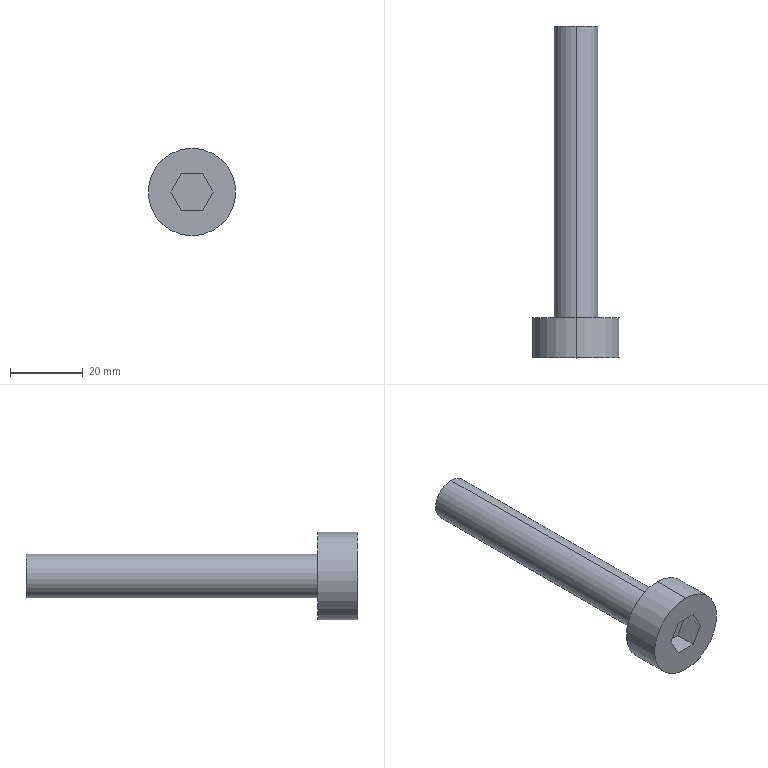Part | STEP file | PN_0057 (M12X60) | 1 solid | 14 faces | box 24 x 91 x 24 mm | volume 13504 mm3 | plane 10 | cylinder 4 | commonest cylinder face diameters 12 x2 24 x2
STEP:
#1=CARTESIAN_POINT('',(0.,0.,0.));
#2=DIRECTION('',(0.,0.,1.));
#3=DIRECTION('',(1.,0.,0.));
#4=AXIS2_PLACEMENT_3D('',#1,#2,#3);
#5=CARTESIAN_POINT('',(0.,91.,-6.));
#6=VERTEX_POINT('',#5);
#7=CARTESIAN_POINT('',(0.,91.,6.));
#8=VERTEX_POINT('',#7);
#9=CARTESIAN_POINT('',(0.,91.,0.));
#10=DIRECTION('',(0.,-1.,0.));
#11=DIRECTION('',(0.,0.,-1.));
#12=AXIS2_PLACEMENT_3D('',#9,#10,#11);
#13=CIRCLE('',#12,6.);
#14=CARTESIAN_POINT('',(0.,0.,0.));
#15=DIRECTION('',(0.,-1.,0.));
#16=DIRECTION('',(0.,0.,-1.));
#17=AXIS2_PLACEMENT_3D('',#14,#15,#16);
#18=CYLINDRICAL_SURFACE('',#17,6.);
#19=CARTESIAN_POINT('',(0.,-91.));
#20=DIRECTION('',(1.,0.));
#21=VECTOR('',#20,1.);
#22=LINE('',#19,#21);
#23=(GEOMETRIC_REPRESENTATION_CONTEXT(2)PARAMETRIC_REPRESENTATION_CONTEXT()REPRESENTATION_CONTEXT('',''));
#24=DEFINITIONAL_REPRESENTATION('',(#22),#23);
#25=PCURVE('',#18,#24);
#26=CARTESIAN_POINT('',(6.,91.,0.));
#27=DIRECTION('',(0.,1.,0.));
#28=DIRECTION('',(0.,0.,1.));
#29=AXIS2_PLACEMENT_3D('',#26,#27,#28);
#30=PLANE('',#29);
#31=CARTESIAN_POINT('',(-6.,-6.));
#32=CARTESIAN_POINT('',(-6.,4.392));
#33=CARTESIAN_POINT('',(3.,-0.8038));
#34=CARTESIAN_POINT('',(12.,-6.));
#35=CARTESIAN_POINT('',(3.,-11.196));
#36=CARTESIAN_POINT('',(-6.,-16.392));
#37=CARTESIAN_POINT('',(-6.,-6.));
#38=(BOUNDED_CURVE()B_SPLINE_CURVE(2,(#31,#32,#33,#34,#35,#36,#37),.UNSPECIFIED.,.T.,.F.)B_SPLINE_CURVE_WITH_KNOTS((1,2,2,2,2,1),(-2.094,0.,2.094,4.189,6.283,8.378),.UNSPECIFIED.)CURVE()GEOMETRIC_REPRESENTATION_ITEM()RATIONAL_B_SPLINE_CURVE((1.,0.5,1.,0.5,1.,0.5,1.))REPRESENTATION_ITEM(''));
#39=(GEOMETRIC_REPRESENTATION_CONTEXT(2)PARAMETRIC_REPRESENTATION_CONTEXT()REPRESENTATION_CONTEXT('',''));
#40=DEFINITIONAL_REPRESENTATION('',(#38),#39);
#41=PCURVE('',#30,#40);
#42=SURFACE_CURVE('',#13,(#25,#41),.PCURVE_S1.);
#43=EDGE_CURVE('',#6,#8,#42,.T.);
#44=ORIENTED_EDGE('',*,*,#43,.T.);
#45=CARTESIAN_POINT('',(0.,11.,6.));
#46=VERTEX_POINT('',#45);
#47=CARTESIAN_POINT('',(0.,0.,6.));
#48=DIRECTION('',(0.,-1.,0.));
#49=VECTOR('',#48,1.);
#50=LINE('',#47,#49);
#51=CARTESIAN_POINT('',(3.142,0.));
#52=DIRECTION('',(0.,1.));
#53=VECTOR('',#52,1.);
#54=LINE('',#51,#53);
#55=(GEOMETRIC_REPRESENTATION_CONTEXT(2)PARAMETRIC_REPRESENTATION_CONTEXT()REPRESENTATION_CONTEXT('',''));
#56=DEFINITIONAL_REPRESENTATION('',(#54),#55);
#57=PCURVE('',#18,#56);
#58=CARTESIAN_POINT('',(0.,0.,0.));
#59=DIRECTION('',(0.,-1.,0.));
#60=DIRECTION('',(0.,0.,-1.));
#61=AXIS2_PLACEMENT_3D('',#58,#59,#60);
#62=CYLINDRICAL_SURFACE('',#61,6.);
#63=CARTESIAN_POINT('',(3.142,0.));
#64=DIRECTION('',(0.,1.));
#65=VECTOR('',#64,1.);
#66=LINE('',#63,#65);
#67=(GEOMETRIC_REPRESENTATION_CONTEXT(2)PARAMETRIC_REPRESENTATION_CONTEXT()REPRESENTATION_CONTEXT('',''));
#68=DEFINITIONAL_REPRESENTATION('',(#66),#67);
#69=PCURVE('',#62,#68);
#70=SURFACE_CURVE('',#50,(#57,#69),.PCURVE_S1.);
#71=EDGE_CURVE('',#8,#46,#70,.T.);
#72=ORIENTED_EDGE('',*,*,#71,.T.);
#73=CARTESIAN_POINT('',(0.,11.,-6.));
#74=VERTEX_POINT('',#73);
#75=CARTESIAN_POINT('',(0.,11.,0.));
#76=DIRECTION('',(0.,-1.,0.));
#77=DIRECTION('',(0.,0.,-1.));
#78=AXIS2_PLACEMENT_3D('',#75,#76,#77);
#79=CIRCLE('',#78,6.);
#80=CARTESIAN_POINT('',(0.,-11.));
#81=DIRECTION('',(1.,0.));
#82=VECTOR('',#81,1.);
#83=LINE('',#80,#82);
#84=(GEOMETRIC_REPRESENTATION_CONTEXT(2)PARAMETRIC_REPRESENTATION_CONTEXT()REPRESENTATION_CONTEXT('',''));
#85=DEFINITIONAL_REPRESENTATION('',(#83),#84);
#86=PCURVE('',#18,#85);
#87=CARTESIAN_POINT('',(12.,11.,0.));
#88=DIRECTION('',(0.,1.,0.));
#89=DIRECTION('',(0.,0.,1.));
#90=AXIS2_PLACEMENT_3D('',#87,#88,#89);
#91=PLANE('',#90);
#92=CARTESIAN_POINT('',(-6.,-12.));
#93=CARTESIAN_POINT('',(-6.,-1.608));
#94=CARTESIAN_POINT('',(3.,-6.804));
#95=CARTESIAN_POINT('',(12.,-12.));
#96=CARTESIAN_POINT('',(3.,-17.196));
#97=CARTESIAN_POINT('',(-6.,-22.392));
#98=CARTESIAN_POINT('',(-6.,-12.));
#99=(BOUNDED_CURVE()B_SPLINE_CURVE(2,(#92,#93,#94,#95,#96,#97,#98),.UNSPECIFIED.,.T.,.F.)B_SPLINE_CURVE_WITH_KNOTS((1,2,2,2,2,1),(-2.094,0.,2.094,4.189,6.283,8.378),.UNSPECIFIED.)CURVE()GEOMETRIC_REPRESENTATION_ITEM()RATIONAL_B_SPLINE_CURVE((1.,0.5,1.,0.5,1.,0.5,1.))REPRESENTATION_ITEM(''));
#100=(GEOMETRIC_REPRESENTATION_CONTEXT(2)PARAMETRIC_REPRESENTATION_CONTEXT()REPRESENTATION_CONTEXT('',''));
#101=DEFINITIONAL_REPRESENTATION('',(#99),#100);
#102=PCURVE('',#91,#101);
#103=SURFACE_CURVE('',#79,(#86,#102),.PCURVE_S1.);
#104=EDGE_CURVE('',#74,#46,#103,.T.);
#105=ORIENTED_EDGE('',*,*,#104,.F.);
#106=CARTESIAN_POINT('',(0.,0.,-6.));
#107=DIRECTION('',(0.,-1.,0.));
#108=VECTOR('',#107,1.);
#109=LINE('',#106,#108);
#110=CARTESIAN_POINT('',(0.,0.));
#111=DIRECTION('',(0.,1.));
#112=VECTOR('',#111,1.);
#113=LINE('',#110,#112);
#114=(GEOMETRIC_REPRESENTATION_CONTEXT(2)PARAMETRIC_REPRESENTATION_CONTEXT()REPRESENTATION_CONTEXT('',''));
#115=DEFINITIONAL_REPRESENTATION('',(#113),#114);
#116=PCURVE('',#18,#115);
#117=CARTESIAN_POINT('',(6.283,0.));
#118=DIRECTION('',(0.,1.));
#119=VECTOR('',#118,1.);
#120=LINE('',#117,#119);
#121=(GEOMETRIC_REPRESENTATION_CONTEXT(2)PARAMETRIC_REPRESENTATION_CONTEXT()REPRESENTATION_CONTEXT('',''));
#122=DEFINITIONAL_REPRESENTATION('',(#120),#121);
#123=PCURVE('',#62,#122);
#124=SURFACE_CURVE('',#109,(#116,#123),.PCURVE_S1.);
#125=EDGE_CURVE('',#6,#74,#124,.T.);
#126=ORIENTED_EDGE('',*,*,#125,.F.);
#127=EDGE_LOOP('',(#44,#72,#105,#126));
#128=FACE_BOUND('',#127,.T.);
#129=ADVANCED_FACE('',(#128),#18,.T.);
#130=CARTESIAN_POINT('',(0.,11.,-12.));
#131=VERTEX_POINT('',#130);
#132=CARTESIAN_POINT('',(0.,11.,12.));
#133=VERTEX_POINT('',#132);
#134=CARTESIAN_POINT('',(0.,11.,0.));
#135=DIRECTION('',(0.,-1.,0.));
#136=DIRECTION('',(0.,0.,-1.));
#137=AXIS2_PLACEMENT_3D('',#134,#135,#136);
#138=CIRCLE('',#137,12.);
#139=CARTESIAN_POINT('',(0.,0.,0.));
#140=DIRECTION('',(0.,-1.,0.));
#141=DIRECTION('',(0.,0.,-1.));
#142=AXIS2_PLACEMENT_3D('',#139,#140,#141);
#143=CYLINDRICAL_SURFACE('',#142,12.);
#144=CARTESIAN_POINT('',(0.,-11.));
#145=DIRECTION('',(1.,0.));
#146=VECTOR('',#145,1.);
#147=LINE('',#144,#146);
#148=(GEOMETRIC_REPRESENTATION_CONTEXT(2)PARAMETRIC_REPRESENTATION_CONTEXT()REPRESENTATION_CONTEXT('',''));
#149=DEFINITIONAL_REPRESENTATION('',(#147),#148);
#150=PCURVE('',#143,#149);
#151=CARTESIAN_POINT('',(-12.,-12.));
#152=CARTESIAN_POINT('',(-12.,8.785));
#153=CARTESIAN_POINT('',(6.,-1.608));
#154=CARTESIAN_POINT('',(24.,-12.));
#155=CARTESIAN_POINT('',(6.,-22.392));
#156=CARTESIAN_POINT('',(-12.,-32.785));
#157=CARTESIAN_POINT('',(-12.,-12.));
#158=(BOUNDED_CURVE()B_SPLINE_CURVE(2,(#151,#152,#153,#154,#155,#156,#157),.UNSPECIFIED.,.T.,.F.)B_SPLINE_CURVE_WITH_KNOTS((1,2,2,2,2,1),(-2.094,0.,2.094,4.189,6.283,8.378),.UNSPECIFIED.)CURVE()GEOMETRIC_REPRESENTATION_ITEM()RATIONAL_B_SPLINE_CURVE((1.,0.5,1.,0.5,1.,0.5,1.))REPRESENTATION_ITEM(''));
#159=(GEOMETRIC_REPRESENTATION_CONTEXT(2)PARAMETRIC_REPRESENTATION_CONTEXT()REPRESENTATION_CONTEXT('',''));
#160=DEFINITIONAL_REPRESENTATION('',(#158),#159);
#161=PCURVE('',#91,#160);
#162=SURFACE_CURVE('',#138,(#150,#161),.PCURVE_S1.);
#163=EDGE_CURVE('',#131,#133,#162,.T.);
#164=ORIENTED_EDGE('',*,*,#163,.T.);
#165=CARTESIAN_POINT('',(0.,0.,12.));
#166=VERTEX_POINT('',#165);
#167=CARTESIAN_POINT('',(0.,0.,12.));
#168=DIRECTION('',(0.,-1.,0.));
#169=VECTOR('',#168,1.);
#170=LINE('',#167,#169);
#171=CARTESIAN_POINT('',(3.142,0.));
#172=DIRECTION('',(0.,1.));
#173=VECTOR('',#172,1.);
#174=LINE('',#171,#173);
#175=(GEOMETRIC_REPRESENTATION_CONTEXT(2)PARAMETRIC_REPRESENTATION_CONTEXT()REPRESENTATION_CONTEXT('',''));
#176=DEFINITIONAL_REPRESENTATION('',(#174),#175);
#177=PCURVE('',#143,#176);
#178=CARTESIAN_POINT('',(0.,0.,0.));
#179=DIRECTION('',(0.,-1.,0.));
#180=DIRECTION('',(0.,0.,-1.));
#181=AXIS2_PLACEMENT_3D('',#178,#179,#180);
#182=CYLINDRICAL_SURFACE('',#181,12.);
#183=CARTESIAN_POINT('',(3.142,0.));
#184=DIRECTION('',(0.,1.));
#185=VECTOR('',#184,1.);
#186=LINE('',#183,#185);
#187=(GEOMETRIC_REPRESENTATION_CONTEXT(2)PARAMETRIC_REPRESENTATION_CONTEXT()REPRESENTATION_CONTEXT('',''));
#188=DEFINITIONAL_REPRESENTATION('',(#186),#187);
#189=PCURVE('',#182,#188);
#190=SURFACE_CURVE('',#170,(#177,#189),.PCURVE_S1.);
#191=EDGE_CURVE('',#133,#166,#190,.T.);
#192=ORIENTED_EDGE('',*,*,#191,.T.);
#193=CARTESIAN_POINT('',(0.,0.,-12.));
#194=VERTEX_POINT('',#193);
#195=CARTESIAN_POINT('',(0.,0.,0.));
#196=DIRECTION('',(0.,-1.,0.));
#197=DIRECTION('',(0.,0.,-1.));
#198=AXIS2_PLACEMENT_3D('',#195,#196,#197);
#199=CIRCLE('',#198,12.);
#200=CARTESIAN_POINT('',(0.,0.));
#201=DIRECTION('',(1.,0.));
#202=VECTOR('',#201,1.);
#203=LINE('',#200,#202);
#204=(GEOMETRIC_REPRESENTATION_CONTEXT(2)PARAMETRIC_REPRESENTATION_CONTEXT()REPRESENTATION_CONTEXT('',''));
#205=DEFINITIONAL_REPRESENTATION('',(#203),#204);
#206=PCURVE('',#143,#205);
#207=CARTESIAN_POINT('',(0.,0.,0.));
#208=DIRECTION('',(0.,-1.,0.));
#209=DIRECTION('',(0.,0.,-1.));
#210=AXIS2_PLACEMENT_3D('',#207,#208,#209);
#211=PLANE('',#210);
#212=CARTESIAN_POINT('',(0.,0.));
#213=DIRECTION('',(1.,0.));
#214=AXIS2_PLACEMENT_2D('',#212,#213);
#215=CIRCLE('',#214,12.);
#216=(GEOMETRIC_REPRESENTATION_CONTEXT(2)PARAMETRIC_REPRESENTATION_CONTEXT()REPRESENTATION_CONTEXT('',''));
#217=DEFINITIONAL_REPRESENTATION('',(#215),#216);
#218=PCURVE('',#211,#217);
#219=SURFACE_CURVE('',#199,(#206,#218),.PCURVE_S1.);
#220=EDGE_CURVE('',#194,#166,#219,.T.);
#221=ORIENTED_EDGE('',*,*,#220,.F.);
#222=CARTESIAN_POINT('',(0.,0.,-12.));
#223=DIRECTION('',(0.,-1.,0.));
#224=VECTOR('',#223,1.);
#225=LINE('',#222,#224);
#226=CARTESIAN_POINT('',(0.,0.));
#227=DIRECTION('',(0.,1.));
#228=VECTOR('',#227,1.);
#229=LINE('',#226,#228);
#230=(GEOMETRIC_REPRESENTATION_CONTEXT(2)PARAMETRIC_REPRESENTATION_CONTEXT()REPRESENTATION_CONTEXT('',''));
#231=DEFINITIONAL_REPRESENTATION('',(#229),#230);
#232=PCURVE('',#143,#231);
#233=CARTESIAN_POINT('',(6.283,0.));
#234=DIRECTION('',(0.,1.));
#235=VECTOR('',#234,1.);
#236=LINE('',#233,#235);
#237=(GEOMETRIC_REPRESENTATION_CONTEXT(2)PARAMETRIC_REPRESENTATION_CONTEXT()REPRESENTATION_CONTEXT('',''));
#238=DEFINITIONAL_REPRESENTATION('',(#236),#237);
#239=PCURVE('',#182,#238);
#240=SURFACE_CURVE('',#225,(#232,#239),.PCURVE_S1.);
#241=EDGE_CURVE('',#131,#194,#240,.T.);
#242=ORIENTED_EDGE('',*,*,#241,.F.);
#243=EDGE_LOOP('',(#164,#192,#221,#242));
#244=FACE_BOUND('',#243,.T.);
#245=ADVANCED_FACE('',(#244),#143,.T.);
#246=CARTESIAN_POINT('',(2.887,0.,-5.));
#247=VERTEX_POINT('',#246);
#248=CARTESIAN_POINT('',(5.774,0.,0.));
#249=VERTEX_POINT('',#248);
#250=CARTESIAN_POINT('',(2.887,0.,-5.));
#251=DIRECTION('',(0.5,0.,0.866));
#252=VECTOR('',#251,1.);
#253=LINE('',#250,#252);
#254=CARTESIAN_POINT('',(5.,2.887));
#255=DIRECTION('',(-0.866,0.5));
#256=VECTOR('',#255,1.);
#257=LINE('',#254,#256);
#258=(GEOMETRIC_REPRESENTATION_CONTEXT(2)PARAMETRIC_REPRESENTATION_CONTEXT()REPRESENTATION_CONTEXT('',''));
#259=DEFINITIONAL_REPRESENTATION('',(#257),#258);
#260=PCURVE('',#211,#259);
#261=CARTESIAN_POINT('',(2.887,6.,-5.));
#262=DIRECTION('',(0.866,0.,-0.5));
#263=DIRECTION('',(-0.5,0.,-0.866));
#264=AXIS2_PLACEMENT_3D('',#261,#262,#263);
#265=PLANE('',#264);
#266=CARTESIAN_POINT('',(0.,-6.));
#267=DIRECTION('',(-1.,0.));
#268=VECTOR('',#267,1.);
#269=LINE('',#266,#268);
#270=(GEOMETRIC_REPRESENTATION_CONTEXT(2)PARAMETRIC_REPRESENTATION_CONTEXT()REPRESENTATION_CONTEXT('',''));
#271=DEFINITIONAL_REPRESENTATION('',(#269),#270);
#272=PCURVE('',#265,#271);
#273=SURFACE_CURVE('',#253,(#260,#272),.PCURVE_S1.);
#274=EDGE_CURVE('',#247,#249,#273,.T.);
#275=ORIENTED_EDGE('',*,*,#274,.F.);
#276=CARTESIAN_POINT('',(-2.887,0.,-5.));
#277=VERTEX_POINT('',#276);
#278=CARTESIAN_POINT('',(-2.887,0.,-5.));
#279=DIRECTION('',(1.,0.,0.));
#280=VECTOR('',#279,1.);
#281=LINE('',#278,#280);
#282=CARTESIAN_POINT('',(5.,-2.887));
#283=DIRECTION('',(0.,1.));
#284=VECTOR('',#283,1.);
#285=LINE('',#282,#284);
#286=(GEOMETRIC_REPRESENTATION_CONTEXT(2)PARAMETRIC_REPRESENTATION_CONTEXT()REPRESENTATION_CONTEXT('',''));
#287=DEFINITIONAL_REPRESENTATION('',(#285),#286);
#288=PCURVE('',#211,#287);
#289=CARTESIAN_POINT('',(-2.887,6.,-5.));
#290=DIRECTION('',(0.,0.,-1.));
#291=DIRECTION('',(-1.,0.,0.));
#292=AXIS2_PLACEMENT_3D('',#289,#290,#291);
#293=PLANE('',#292);
#294=CARTESIAN_POINT('',(0.,-6.));
#295=DIRECTION('',(-1.,0.));
#296=VECTOR('',#295,1.);
#297=LINE('',#294,#296);
#298=(GEOMETRIC_REPRESENTATION_CONTEXT(2)PARAMETRIC_REPRESENTATION_CONTEXT()REPRESENTATION_CONTEXT('',''));
#299=DEFINITIONAL_REPRESENTATION('',(#297),#298);
#300=PCURVE('',#293,#299);
#301=SURFACE_CURVE('',#281,(#288,#300),.PCURVE_S1.);
#302=EDGE_CURVE('',#277,#247,#301,.T.);
#303=ORIENTED_EDGE('',*,*,#302,.F.);
#304=CARTESIAN_POINT('',(-5.774,0.,0.));
#305=VERTEX_POINT('',#304);
#306=CARTESIAN_POINT('',(-5.774,0.,0.));
#307=DIRECTION('',(0.5,0.,-0.866));
#308=VECTOR('',#307,1.);
#309=LINE('',#306,#308);
#310=CARTESIAN_POINT('',(0.,-5.774));
#311=DIRECTION('',(0.866,0.5));
#312=VECTOR('',#311,1.);
#313=LINE('',#310,#312);
#314=(GEOMETRIC_REPRESENTATION_CONTEXT(2)PARAMETRIC_REPRESENTATION_CONTEXT()REPRESENTATION_CONTEXT('',''));
#315=DEFINITIONAL_REPRESENTATION('',(#313),#314);
#316=PCURVE('',#211,#315);
#317=CARTESIAN_POINT('',(-5.774,6.,0.));
#318=DIRECTION('',(-0.866,0.,-0.5));
#319=DIRECTION('',(-0.5,0.,0.866));
#320=AXIS2_PLACEMENT_3D('',#317,#318,#319);
#321=PLANE('',#320);
#322=CARTESIAN_POINT('',(0.,-6.));
#323=DIRECTION('',(-1.,0.));
#324=VECTOR('',#323,1.);
#325=LINE('',#322,#324);
#326=(GEOMETRIC_REPRESENTATION_CONTEXT(2)PARAMETRIC_REPRESENTATION_CONTEXT()REPRESENTATION_CONTEXT('',''));
#327=DEFINITIONAL_REPRESENTATION('',(#325),#326);
#328=PCURVE('',#321,#327);
#329=SURFACE_CURVE('',#309,(#316,#328),.PCURVE_S1.);
#330=EDGE_CURVE('',#305,#277,#329,.T.);
#331=ORIENTED_EDGE('',*,*,#330,.F.);
#332=CARTESIAN_POINT('',(-2.887,0.,5.));
#333=VERTEX_POINT('',#332);
#334=CARTESIAN_POINT('',(-2.887,0.,5.));
#335=DIRECTION('',(-0.5,0.,-0.866));
#336=VECTOR('',#335,1.);
#337=LINE('',#334,#336);
#338=CARTESIAN_POINT('',(-5.,-2.887));
#339=DIRECTION('',(0.866,-0.5));
#340=VECTOR('',#339,1.);
#341=LINE('',#338,#340);
#342=(GEOMETRIC_REPRESENTATION_CONTEXT(2)PARAMETRIC_REPRESENTATION_CONTEXT()REPRESENTATION_CONTEXT('',''));
#343=DEFINITIONAL_REPRESENTATION('',(#341),#342);
#344=PCURVE('',#211,#343);
#345=CARTESIAN_POINT('',(-2.887,6.,5.));
#346=DIRECTION('',(-0.866,0.,0.5));
#347=DIRECTION('',(0.5,0.,0.866));
#348=AXIS2_PLACEMENT_3D('',#345,#346,#347);
#349=PLANE('',#348);
#350=CARTESIAN_POINT('',(0.,-6.));
#351=DIRECTION('',(-1.,0.));
#352=VECTOR('',#351,1.);
#353=LINE('',#350,#352);
#354=(GEOMETRIC_REPRESENTATION_CONTEXT(2)PARAMETRIC_REPRESENTATION_CONTEXT()REPRESENTATION_CONTEXT('',''));
#355=DEFINITIONAL_REPRESENTATION('',(#353),#354);
#356=PCURVE('',#349,#355);
#357=SURFACE_CURVE('',#337,(#344,#356),.PCURVE_S1.);
#358=EDGE_CURVE('',#333,#305,#357,.T.);
#359=ORIENTED_EDGE('',*,*,#358,.F.);
#360=CARTESIAN_POINT('',(2.887,0.,5.));
#361=VERTEX_POINT('',#360);
#362=CARTESIAN_POINT('',(2.887,0.,5.));
#363=DIRECTION('',(-1.,0.,0.));
#364=VECTOR('',#363,1.);
#365=LINE('',#362,#364);
#366=CARTESIAN_POINT('',(-5.,2.887));
#367=DIRECTION('',(0.,-1.));
#368=VECTOR('',#367,1.);
#369=LINE('',#366,#368);
#370=(GEOMETRIC_REPRESENTATION_CONTEXT(2)PARAMETRIC_REPRESENTATION_CONTEXT()REPRESENTATION_CONTEXT('',''));
#371=DEFINITIONAL_REPRESENTATION('',(#369),#370);
#372=PCURVE('',#211,#371);
#373=CARTESIAN_POINT('',(2.887,6.,5.));
#374=DIRECTION('',(0.,0.,1.));
#375=DIRECTION('',(1.,0.,0.));
#376=AXIS2_PLACEMENT_3D('',#373,#374,#375);
#377=PLANE('',#376);
#378=CARTESIAN_POINT('',(0.,-6.));
#379=DIRECTION('',(-1.,0.));
#380=VECTOR('',#379,1.);
#381=LINE('',#378,#380);
#382=(GEOMETRIC_REPRESENTATION_CONTEXT(2)PARAMETRIC_REPRESENTATION_CONTEXT()REPRESENTATION_CONTEXT('',''));
#383=DEFINITIONAL_REPRESENTATION('',(#381),#382);
#384=PCURVE('',#377,#383);
#385=SURFACE_CURVE('',#365,(#372,#384),.PCURVE_S1.);
#386=EDGE_CURVE('',#361,#333,#385,.T.);
#387=ORIENTED_EDGE('',*,*,#386,.F.);
#388=CARTESIAN_POINT('',(5.774,0.,0.));
#389=DIRECTION('',(-0.5,0.,0.866));
#390=VECTOR('',#389,1.);
#391=LINE('',#388,#390);
#392=CARTESIAN_POINT('',(0.,5.774));
#393=DIRECTION('',(-0.866,-0.5));
#394=VECTOR('',#393,1.);
#395=LINE('',#392,#394);
#396=(GEOMETRIC_REPRESENTATION_CONTEXT(2)PARAMETRIC_REPRESENTATION_CONTEXT()REPRESENTATION_CONTEXT('',''));
#397=DEFINITIONAL_REPRESENTATION('',(#395),#396);
#398=PCURVE('',#211,#397);
#399=CARTESIAN_POINT('',(5.774,6.,0.));
#400=DIRECTION('',(0.866,0.,0.5));
#401=DIRECTION('',(0.5,0.,-0.866));
#402=AXIS2_PLACEMENT_3D('',#399,#400,#401);
#403=PLANE('',#402);
#404=CARTESIAN_POINT('',(0.,-6.));
#405=DIRECTION('',(-1.,0.));
#406=VECTOR('',#405,1.);
#407=LINE('',#404,#406);
#408=(GEOMETRIC_REPRESENTATION_CONTEXT(2)PARAMETRIC_REPRESENTATION_CONTEXT()REPRESENTATION_CONTEXT('',''));
#409=DEFINITIONAL_REPRESENTATION('',(#407),#408);
#410=PCURVE('',#403,#409);
#411=SURFACE_CURVE('',#391,(#398,#410),.PCURVE_S1.);
#412=EDGE_CURVE('',#249,#361,#411,.T.);
#413=ORIENTED_EDGE('',*,*,#412,.F.);
#414=EDGE_LOOP('',(#275,#303,#331,#359,#387,#413));
#415=FACE_BOUND('',#414,.T.);
#416=ORIENTED_EDGE('',*,*,#220,.T.);
#417=CARTESIAN_POINT('',(0.,0.,0.));
#418=DIRECTION('',(0.,-1.,0.));
#419=DIRECTION('',(0.,0.,-1.));
#420=AXIS2_PLACEMENT_3D('',#417,#418,#419);
#421=CIRCLE('',#420,12.);
#422=CARTESIAN_POINT('',(0.,0.));
#423=DIRECTION('',(1.,0.));
#424=AXIS2_PLACEMENT_2D('',#422,#423);
#425=CIRCLE('',#424,12.);
#426=(GEOMETRIC_REPRESENTATION_CONTEXT(2)PARAMETRIC_REPRESENTATION_CONTEXT()REPRESENTATION_CONTEXT('',''));
#427=DEFINITIONAL_REPRESENTATION('',(#425),#426);
#428=PCURVE('',#211,#427);
#429=CARTESIAN_POINT('',(0.,0.));
#430=DIRECTION('',(1.,0.));
#431=VECTOR('',#430,1.);
#432=LINE('',#429,#431);
#433=(GEOMETRIC_REPRESENTATION_CONTEXT(2)PARAMETRIC_REPRESENTATION_CONTEXT()REPRESENTATION_CONTEXT('',''));
#434=DEFINITIONAL_REPRESENTATION('',(#432),#433);
#435=PCURVE('',#182,#434);
#436=SURFACE_CURVE('',#421,(#428,#435),.PCURVE_S1.);
#437=EDGE_CURVE('',#166,#194,#436,.T.);
#438=ORIENTED_EDGE('',*,*,#437,.T.);
#439=EDGE_LOOP('',(#416,#438));
#440=FACE_BOUND('',#439,.T.);
#441=ADVANCED_FACE('',(#415,#440),#211,.T.);
#442=ORIENTED_EDGE('',*,*,#191,.F.);
#443=CARTESIAN_POINT('',(0.,11.,0.));
#444=DIRECTION('',(0.,-1.,0.));
#445=DIRECTION('',(0.,0.,-1.));
#446=AXIS2_PLACEMENT_3D('',#443,#444,#445);
#447=CIRCLE('',#446,12.);
#448=CARTESIAN_POINT('',(0.,-11.));
#449=DIRECTION('',(1.,0.));
#450=VECTOR('',#449,1.);
#451=LINE('',#448,#450);
#452=(GEOMETRIC_REPRESENTATION_CONTEXT(2)PARAMETRIC_REPRESENTATION_CONTEXT()REPRESENTATION_CONTEXT('',''));
#453=DEFINITIONAL_REPRESENTATION('',(#451),#452);
#454=PCURVE('',#182,#453);
#455=CARTESIAN_POINT('',(-12.,-12.));
#456=CARTESIAN_POINT('',(-12.,8.785));
#457=CARTESIAN_POINT('',(6.,-1.608));
#458=CARTESIAN_POINT('',(24.,-12.));
#459=CARTESIAN_POINT('',(6.,-22.392));
#460=CARTESIAN_POINT('',(-12.,-32.785));
#461=CARTESIAN_POINT('',(-12.,-12.));
#462=(BOUNDED_CURVE()B_SPLINE_CURVE(2,(#455,#456,#457,#458,#459,#460,#461),.UNSPECIFIED.,.T.,.F.)B_SPLINE_CURVE_WITH_KNOTS((1,2,2,2,2,1),(-2.094,0.,2.094,4.189,6.283,8.378),.UNSPECIFIED.)CURVE()GEOMETRIC_REPRESENTATION_ITEM()RATIONAL_B_SPLINE_CURVE((1.,0.5,1.,0.5,1.,0.5,1.))REPRESENTATION_ITEM(''));
#463=(GEOMETRIC_REPRESENTATION_CONTEXT(2)PARAMETRIC_REPRESENTATION_CONTEXT()REPRESENTATION_CONTEXT('',''));
#464=DEFINITIONAL_REPRESENTATION('',(#462),#463);
#465=PCURVE('',#91,#464);
#466=SURFACE_CURVE('',#447,(#454,#465),.PCURVE_S1.);
#467=EDGE_CURVE('',#133,#131,#466,.T.);
#468=ORIENTED_EDGE('',*,*,#467,.T.);
#469=ORIENTED_EDGE('',*,*,#241,.T.);
#470=ORIENTED_EDGE('',*,*,#437,.F.);
#471=EDGE_LOOP('',(#442,#468,#469,#470));
#472=FACE_BOUND('',#471,.T.);
#473=ADVANCED_FACE('',(#472),#182,.T.);
#474=ORIENTED_EDGE('',*,*,#104,.T.);
#475=CARTESIAN_POINT('',(0.,11.,0.));
#476=DIRECTION('',(0.,-1.,0.));
#477=DIRECTION('',(0.,0.,-1.));
#478=AXIS2_PLACEMENT_3D('',#475,#476,#477);
#479=CIRCLE('',#478,6.);
#480=CARTESIAN_POINT('',(-6.,-12.));
#481=CARTESIAN_POINT('',(-6.,-1.608));
#482=CARTESIAN_POINT('',(3.,-6.804));
#483=CARTESIAN_POINT('',(12.,-12.));
#484=CARTESIAN_POINT('',(3.,-17.196));
#485=CARTESIAN_POINT('',(-6.,-22.392));
#486=CARTESIAN_POINT('',(-6.,-12.));
#487=(BOUNDED_CURVE()B_SPLINE_CURVE(2,(#480,#481,#482,#483,#484,#485,#486),.UNSPECIFIED.,.T.,.F.)B_SPLINE_CURVE_WITH_KNOTS((1,2,2,2,2,1),(-2.094,0.,2.094,4.189,6.283,8.378),.UNSPECIFIED.)CURVE()GEOMETRIC_REPRESENTATION_ITEM()RATIONAL_B_SPLINE_CURVE((1.,0.5,1.,0.5,1.,0.5,1.))REPRESENTATION_ITEM(''));
#488=(GEOMETRIC_REPRESENTATION_CONTEXT(2)PARAMETRIC_REPRESENTATION_CONTEXT()REPRESENTATION_CONTEXT('',''));
#489=DEFINITIONAL_REPRESENTATION('',(#487),#488);
#490=PCURVE('',#91,#489);
#491=CARTESIAN_POINT('',(0.,-11.));
#492=DIRECTION('',(1.,0.));
#493=VECTOR('',#492,1.);
#494=LINE('',#491,#493);
#495=(GEOMETRIC_REPRESENTATION_CONTEXT(2)PARAMETRIC_REPRESENTATION_CONTEXT()REPRESENTATION_CONTEXT('',''));
#496=DEFINITIONAL_REPRESENTATION('',(#494),#495);
#497=PCURVE('',#62,#496);
#498=SURFACE_CURVE('',#479,(#490,#497),.PCURVE_S1.);
#499=EDGE_CURVE('',#46,#74,#498,.T.);
#500=ORIENTED_EDGE('',*,*,#499,.T.);
#501=EDGE_LOOP('',(#474,#500));
#502=FACE_BOUND('',#501,.T.);
#503=ORIENTED_EDGE('',*,*,#163,.F.);
#504=ORIENTED_EDGE('',*,*,#467,.F.);
#505=EDGE_LOOP('',(#503,#504));
#506=FACE_BOUND('',#505,.T.);
#507=ADVANCED_FACE('',(#502,#506),#91,.T.);
#508=ORIENTED_EDGE('',*,*,#71,.F.);
#509=CARTESIAN_POINT('',(0.,91.,0.));
#510=DIRECTION('',(0.,-1.,0.));
#511=DIRECTION('',(0.,0.,-1.));
#512=AXIS2_PLACEMENT_3D('',#509,#510,#511);
#513=CIRCLE('',#512,6.);
#514=CARTESIAN_POINT('',(0.,-91.));
#515=DIRECTION('',(1.,0.));
#516=VECTOR('',#515,1.);
#517=LINE('',#514,#516);
#518=(GEOMETRIC_REPRESENTATION_CONTEXT(2)PARAMETRIC_REPRESENTATION_CONTEXT()REPRESENTATION_CONTEXT('',''));
#519=DEFINITIONAL_REPRESENTATION('',(#517),#518);
#520=PCURVE('',#62,#519);
#521=CARTESIAN_POINT('',(-6.,-6.));
#522=CARTESIAN_POINT('',(-6.,4.392));
#523=CARTESIAN_POINT('',(3.,-0.8038));
#524=CARTESIAN_POINT('',(12.,-6.));
#525=CARTESIAN_POINT('',(3.,-11.196));
#526=CARTESIAN_POINT('',(-6.,-16.392));
#527=CARTESIAN_POINT('',(-6.,-6.));
#528=(BOUNDED_CURVE()B_SPLINE_CURVE(2,(#521,#522,#523,#524,#525,#526,#527),.UNSPECIFIED.,.T.,.F.)B_SPLINE_CURVE_WITH_KNOTS((1,2,2,2,2,1),(-2.094,0.,2.094,4.189,6.283,8.378),.UNSPECIFIED.)CURVE()GEOMETRIC_REPRESENTATION_ITEM()RATIONAL_B_SPLINE_CURVE((1.,0.5,1.,0.5,1.,0.5,1.))REPRESENTATION_ITEM(''));
#529=(GEOMETRIC_REPRESENTATION_CONTEXT(2)PARAMETRIC_REPRESENTATION_CONTEXT()REPRESENTATION_CONTEXT('',''));
#530=DEFINITIONAL_REPRESENTATION('',(#528),#529);
#531=PCURVE('',#30,#530);
#532=SURFACE_CURVE('',#513,(#520,#531),.PCURVE_S1.);
#533=EDGE_CURVE('',#8,#6,#532,.T.);
#534=ORIENTED_EDGE('',*,*,#533,.T.);
#535=ORIENTED_EDGE('',*,*,#125,.T.);
#536=ORIENTED_EDGE('',*,*,#499,.F.);
#537=EDGE_LOOP('',(#508,#534,#535,#536));
#538=FACE_BOUND('',#537,.T.);
#539=ADVANCED_FACE('',(#538),#62,.T.);
#540=ORIENTED_EDGE('',*,*,#43,.F.);
#541=ORIENTED_EDGE('',*,*,#533,.F.);
#542=EDGE_LOOP('',(#540,#541));
#543=FACE_BOUND('',#542,.T.);
#544=ADVANCED_FACE('',(#543),#30,.T.);
#545=ORIENTED_EDGE('',*,*,#274,.T.);
#546=CARTESIAN_POINT('',(5.774,6.,0.));
#547=VERTEX_POINT('',#546);
#548=CARTESIAN_POINT('',(5.774,6.,0.));
#549=DIRECTION('',(0.,-1.,0.));
#550=VECTOR('',#549,1.);
#551=LINE('',#548,#550);
#552=CARTESIAN_POINT('',(-5.774,0.));
#553=DIRECTION('',(0.,-1.));
#554=VECTOR('',#553,1.);
#555=LINE('',#552,#554);
#556=(GEOMETRIC_REPRESENTATION_CONTEXT(2)PARAMETRIC_REPRESENTATION_CONTEXT()REPRESENTATION_CONTEXT('',''));
#557=DEFINITIONAL_REPRESENTATION('',(#555),#556);
#558=PCURVE('',#265,#557);
#559=CARTESIAN_POINT('',(0.,0.));
#560=DIRECTION('',(0.,-1.));
#561=VECTOR('',#560,1.);
#562=LINE('',#559,#561);
#563=(GEOMETRIC_REPRESENTATION_CONTEXT(2)PARAMETRIC_REPRESENTATION_CONTEXT()REPRESENTATION_CONTEXT('',''));
#564=DEFINITIONAL_REPRESENTATION('',(#562),#563);
#565=PCURVE('',#403,#564);
#566=SURFACE_CURVE('',#551,(#558,#565),.PCURVE_S1.);
#567=EDGE_CURVE('',#547,#249,#566,.T.);
#568=ORIENTED_EDGE('',*,*,#567,.F.);
#569=CARTESIAN_POINT('',(2.887,6.,-5.));
#570=VERTEX_POINT('',#569);
#571=CARTESIAN_POINT('',(2.887,6.,-5.));
#572=DIRECTION('',(0.5,0.,0.866));
#573=VECTOR('',#572,1.);
#574=LINE('',#571,#573);
#575=CARTESIAN_POINT('',(0.,0.));
#576=DIRECTION('',(-1.,0.));
#577=VECTOR('',#576,1.);
#578=LINE('',#575,#577);
#579=(GEOMETRIC_REPRESENTATION_CONTEXT(2)PARAMETRIC_REPRESENTATION_CONTEXT()REPRESENTATION_CONTEXT('',''));
#580=DEFINITIONAL_REPRESENTATION('',(#578),#579);
#581=PCURVE('',#265,#580);
#582=CARTESIAN_POINT('',(0.,6.,0.));
#583=DIRECTION('',(0.,-1.,0.));
#584=DIRECTION('',(0.,0.,-1.));
#585=AXIS2_PLACEMENT_3D('',#582,#583,#584);
#586=PLANE('',#585);
#587=CARTESIAN_POINT('',(5.,2.887));
#588=DIRECTION('',(-0.866,0.5));
#589=VECTOR('',#588,1.);
#590=LINE('',#587,#589);
#591=(GEOMETRIC_REPRESENTATION_CONTEXT(2)PARAMETRIC_REPRESENTATION_CONTEXT()REPRESENTATION_CONTEXT('',''));
#592=DEFINITIONAL_REPRESENTATION('',(#590),#591);
#593=PCURVE('',#586,#592);
#594=SURFACE_CURVE('',#574,(#581,#593),.PCURVE_S1.);
#595=EDGE_CURVE('',#570,#547,#594,.T.);
#596=ORIENTED_EDGE('',*,*,#595,.F.);
#597=CARTESIAN_POINT('',(2.887,6.,-5.));
#598=DIRECTION('',(0.,-1.,0.));
#599=VECTOR('',#598,1.);
#600=LINE('',#597,#599);
#601=CARTESIAN_POINT('',(0.,0.));
#602=DIRECTION('',(0.,-1.));
#603=VECTOR('',#602,1.);
#604=LINE('',#601,#603);
#605=(GEOMETRIC_REPRESENTATION_CONTEXT(2)PARAMETRIC_REPRESENTATION_CONTEXT()REPRESENTATION_CONTEXT('',''));
#606=DEFINITIONAL_REPRESENTATION('',(#604),#605);
#607=PCURVE('',#265,#606);
#608=CARTESIAN_POINT('',(-5.774,0.));
#609=DIRECTION('',(0.,-1.));
#610=VECTOR('',#609,1.);
#611=LINE('',#608,#610);
#612=(GEOMETRIC_REPRESENTATION_CONTEXT(2)PARAMETRIC_REPRESENTATION_CONTEXT()REPRESENTATION_CONTEXT('',''));
#613=DEFINITIONAL_REPRESENTATION('',(#611),#612);
#614=PCURVE('',#293,#613);
#615=SURFACE_CURVE('',#600,(#607,#614),.PCURVE_S1.);
#616=EDGE_CURVE('',#570,#247,#615,.T.);
#617=ORIENTED_EDGE('',*,*,#616,.T.);
#618=EDGE_LOOP('',(#545,#568,#596,#617));
#619=FACE_BOUND('',#618,.T.);
#620=ADVANCED_FACE('',(#619),#265,.F.);
#621=ORIENTED_EDGE('',*,*,#302,.T.);
#622=ORIENTED_EDGE('',*,*,#616,.F.);
#623=CARTESIAN_POINT('',(-2.887,6.,-5.));
#624=VERTEX_POINT('',#623);
#625=CARTESIAN_POINT('',(-2.887,6.,-5.));
#626=DIRECTION('',(1.,0.,0.));
#627=VECTOR('',#626,1.);
#628=LINE('',#625,#627);
#629=CARTESIAN_POINT('',(0.,0.));
#630=DIRECTION('',(-1.,0.));
#631=VECTOR('',#630,1.);
#632=LINE('',#629,#631);
#633=(GEOMETRIC_REPRESENTATION_CONTEXT(2)PARAMETRIC_REPRESENTATION_CONTEXT()REPRESENTATION_CONTEXT('',''));
#634=DEFINITIONAL_REPRESENTATION('',(#632),#633);
#635=PCURVE('',#293,#634);
#636=CARTESIAN_POINT('',(5.,-2.887));
#637=DIRECTION('',(0.,1.));
#638=VECTOR('',#637,1.);
#639=LINE('',#636,#638);
#640=(GEOMETRIC_REPRESENTATION_CONTEXT(2)PARAMETRIC_REPRESENTATION_CONTEXT()REPRESENTATION_CONTEXT('',''));
#641=DEFINITIONAL_REPRESENTATION('',(#639),#640);
#642=PCURVE('',#586,#641);
#643=SURFACE_CURVE('',#628,(#635,#642),.PCURVE_S1.);
#644=EDGE_CURVE('',#624,#570,#643,.T.);
#645=ORIENTED_EDGE('',*,*,#644,.F.);
#646=CARTESIAN_POINT('',(-2.887,6.,-5.));
#647=DIRECTION('',(0.,-1.,0.));
#648=VECTOR('',#647,1.);
#649=LINE('',#646,#648);
#650=CARTESIAN_POINT('',(0.,0.));
#651=DIRECTION('',(0.,-1.));
#652=VECTOR('',#651,1.);
#653=LINE('',#650,#652);
#654=(GEOMETRIC_REPRESENTATION_CONTEXT(2)PARAMETRIC_REPRESENTATION_CONTEXT()REPRESENTATION_CONTEXT('',''));
#655=DEFINITIONAL_REPRESENTATION('',(#653),#654);
#656=PCURVE('',#293,#655);
#657=CARTESIAN_POINT('',(-5.774,0.));
#658=DIRECTION('',(0.,-1.));
#659=VECTOR('',#658,1.);
#660=LINE('',#657,#659);
#661=(GEOMETRIC_REPRESENTATION_CONTEXT(2)PARAMETRIC_REPRESENTATION_CONTEXT()REPRESENTATION_CONTEXT('',''));
#662=DEFINITIONAL_REPRESENTATION('',(#660),#661);
#663=PCURVE('',#321,#662);
#664=SURFACE_CURVE('',#649,(#656,#663),.PCURVE_S1.);
#665=EDGE_CURVE('',#624,#277,#664,.T.);
#666=ORIENTED_EDGE('',*,*,#665,.T.);
#667=EDGE_LOOP('',(#621,#622,#645,#666));
#668=FACE_BOUND('',#667,.T.);
#669=ADVANCED_FACE('',(#668),#293,.F.);
#670=ORIENTED_EDGE('',*,*,#330,.T.);
#671=ORIENTED_EDGE('',*,*,#665,.F.);
#672=CARTESIAN_POINT('',(-5.774,6.,0.));
#673=VERTEX_POINT('',#672);
#674=CARTESIAN_POINT('',(-5.774,6.,0.));
#675=DIRECTION('',(0.5,0.,-0.866));
#676=VECTOR('',#675,1.);
#677=LINE('',#674,#676);
#678=CARTESIAN_POINT('',(0.,0.));
#679=DIRECTION('',(-1.,0.));
#680=VECTOR('',#679,1.);
#681=LINE('',#678,#680);
#682=(GEOMETRIC_REPRESENTATION_CONTEXT(2)PARAMETRIC_REPRESENTATION_CONTEXT()REPRESENTATION_CONTEXT('',''));
#683=DEFINITIONAL_REPRESENTATION('',(#681),#682);
#684=PCURVE('',#321,#683);
#685=CARTESIAN_POINT('',(0.,-5.774));
#686=DIRECTION('',(0.866,0.5));
#687=VECTOR('',#686,1.);
#688=LINE('',#685,#687);
#689=(GEOMETRIC_REPRESENTATION_CONTEXT(2)PARAMETRIC_REPRESENTATION_CONTEXT()REPRESENTATION_CONTEXT('',''));
#690=DEFINITIONAL_REPRESENTATION('',(#688),#689);
#691=PCURVE('',#586,#690);
#692=SURFACE_CURVE('',#677,(#684,#691),.PCURVE_S1.);
#693=EDGE_CURVE('',#673,#624,#692,.T.);
#694=ORIENTED_EDGE('',*,*,#693,.F.);
#695=CARTESIAN_POINT('',(-5.774,6.,0.));
#696=DIRECTION('',(0.,-1.,0.));
#697=VECTOR('',#696,1.);
#698=LINE('',#695,#697);
#699=CARTESIAN_POINT('',(0.,0.));
#700=DIRECTION('',(0.,-1.));
#701=VECTOR('',#700,1.);
#702=LINE('',#699,#701);
#703=(GEOMETRIC_REPRESENTATION_CONTEXT(2)PARAMETRIC_REPRESENTATION_CONTEXT()REPRESENTATION_CONTEXT('',''));
#704=DEFINITIONAL_REPRESENTATION('',(#702),#703);
#705=PCURVE('',#321,#704);
#706=CARTESIAN_POINT('',(-5.774,0.));
#707=DIRECTION('',(0.,-1.));
#708=VECTOR('',#707,1.);
#709=LINE('',#706,#708);
#710=(GEOMETRIC_REPRESENTATION_CONTEXT(2)PARAMETRIC_REPRESENTATION_CONTEXT()REPRESENTATION_CONTEXT('',''));
#711=DEFINITIONAL_REPRESENTATION('',(#709),#710);
#712=PCURVE('',#349,#711);
#713=SURFACE_CURVE('',#698,(#705,#712),.PCURVE_S1.);
#714=EDGE_CURVE('',#673,#305,#713,.T.);
#715=ORIENTED_EDGE('',*,*,#714,.T.);
#716=EDGE_LOOP('',(#670,#671,#694,#715));
#717=FACE_BOUND('',#716,.T.);
#718=ADVANCED_FACE('',(#717),#321,.F.);
#719=ORIENTED_EDGE('',*,*,#358,.T.);
#720=ORIENTED_EDGE('',*,*,#714,.F.);
#721=CARTESIAN_POINT('',(-2.887,6.,5.));
#722=VERTEX_POINT('',#721);
#723=CARTESIAN_POINT('',(-2.887,6.,5.));
#724=DIRECTION('',(-0.5,0.,-0.866));
#725=VECTOR('',#724,1.);
#726=LINE('',#723,#725);
#727=CARTESIAN_POINT('',(0.,0.));
#728=DIRECTION('',(-1.,0.));
#729=VECTOR('',#728,1.);
#730=LINE('',#727,#729);
#731=(GEOMETRIC_REPRESENTATION_CONTEXT(2)PARAMETRIC_REPRESENTATION_CONTEXT()REPRESENTATION_CONTEXT('',''));
#732=DEFINITIONAL_REPRESENTATION('',(#730),#731);
#733=PCURVE('',#349,#732);
#734=CARTESIAN_POINT('',(-5.,-2.887));
#735=DIRECTION('',(0.866,-0.5));
#736=VECTOR('',#735,1.);
#737=LINE('',#734,#736);
#738=(GEOMETRIC_REPRESENTATION_CONTEXT(2)PARAMETRIC_REPRESENTATION_CONTEXT()REPRESENTATION_CONTEXT('',''));
#739=DEFINITIONAL_REPRESENTATION('',(#737),#738);
#740=PCURVE('',#586,#739);
#741=SURFACE_CURVE('',#726,(#733,#740),.PCURVE_S1.);
#742=EDGE_CURVE('',#722,#673,#741,.T.);
#743=ORIENTED_EDGE('',*,*,#742,.F.);
#744=CARTESIAN_POINT('',(-2.887,6.,5.));
#745=DIRECTION('',(0.,-1.,0.));
#746=VECTOR('',#745,1.);
#747=LINE('',#744,#746);
#748=CARTESIAN_POINT('',(0.,0.));
#749=DIRECTION('',(0.,-1.));
#750=VECTOR('',#749,1.);
#751=LINE('',#748,#750);
#752=(GEOMETRIC_REPRESENTATION_CONTEXT(2)PARAMETRIC_REPRESENTATION_CONTEXT()REPRESENTATION_CONTEXT('',''));
#753=DEFINITIONAL_REPRESENTATION('',(#751),#752);
#754=PCURVE('',#349,#753);
#755=CARTESIAN_POINT('',(-5.774,0.));
#756=DIRECTION('',(0.,-1.));
#757=VECTOR('',#756,1.);
#758=LINE('',#755,#757);
#759=(GEOMETRIC_REPRESENTATION_CONTEXT(2)PARAMETRIC_REPRESENTATION_CONTEXT()REPRESENTATION_CONTEXT('',''));
#760=DEFINITIONAL_REPRESENTATION('',(#758),#759);
#761=PCURVE('',#377,#760);
#762=SURFACE_CURVE('',#747,(#754,#761),.PCURVE_S1.);
#763=EDGE_CURVE('',#722,#333,#762,.T.);
#764=ORIENTED_EDGE('',*,*,#763,.T.);
#765=EDGE_LOOP('',(#719,#720,#743,#764));
#766=FACE_BOUND('',#765,.T.);
#767=ADVANCED_FACE('',(#766),#349,.F.);
#768=ORIENTED_EDGE('',*,*,#386,.T.);
#769=ORIENTED_EDGE('',*,*,#763,.F.);
#770=CARTESIAN_POINT('',(2.887,6.,5.));
#771=VERTEX_POINT('',#770);
#772=CARTESIAN_POINT('',(2.887,6.,5.));
#773=DIRECTION('',(-1.,0.,0.));
#774=VECTOR('',#773,1.);
#775=LINE('',#772,#774);
#776=CARTESIAN_POINT('',(0.,0.));
#777=DIRECTION('',(-1.,0.));
#778=VECTOR('',#777,1.);
#779=LINE('',#776,#778);
#780=(GEOMETRIC_REPRESENTATION_CONTEXT(2)PARAMETRIC_REPRESENTATION_CONTEXT()REPRESENTATION_CONTEXT('',''));
#781=DEFINITIONAL_REPRESENTATION('',(#779),#780);
#782=PCURVE('',#377,#781);
#783=CARTESIAN_POINT('',(-5.,2.887));
#784=DIRECTION('',(0.,-1.));
#785=VECTOR('',#784,1.);
#786=LINE('',#783,#785);
#787=(GEOMETRIC_REPRESENTATION_CONTEXT(2)PARAMETRIC_REPRESENTATION_CONTEXT()REPRESENTATION_CONTEXT('',''));
#788=DEFINITIONAL_REPRESENTATION('',(#786),#787);
#789=PCURVE('',#586,#788);
#790=SURFACE_CURVE('',#775,(#782,#789),.PCURVE_S1.);
#791=EDGE_CURVE('',#771,#722,#790,.T.);
#792=ORIENTED_EDGE('',*,*,#791,.F.);
#793=CARTESIAN_POINT('',(2.887,6.,5.));
#794=DIRECTION('',(0.,-1.,0.));
#795=VECTOR('',#794,1.);
#796=LINE('',#793,#795);
#797=CARTESIAN_POINT('',(0.,0.));
#798=DIRECTION('',(0.,-1.));
#799=VECTOR('',#798,1.);
#800=LINE('',#797,#799);
#801=(GEOMETRIC_REPRESENTATION_CONTEXT(2)PARAMETRIC_REPRESENTATION_CONTEXT()REPRESENTATION_CONTEXT('',''));
#802=DEFINITIONAL_REPRESENTATION('',(#800),#801);
#803=PCURVE('',#377,#802);
#804=CARTESIAN_POINT('',(-5.774,0.));
#805=DIRECTION('',(0.,-1.));
#806=VECTOR('',#805,1.);
#807=LINE('',#804,#806);
#808=(GEOMETRIC_REPRESENTATION_CONTEXT(2)PARAMETRIC_REPRESENTATION_CONTEXT()REPRESENTATION_CONTEXT('',''));
#809=DEFINITIONAL_REPRESENTATION('',(#807),#808);
#810=PCURVE('',#403,#809);
#811=SURFACE_CURVE('',#796,(#803,#810),.PCURVE_S1.);
#812=EDGE_CURVE('',#771,#361,#811,.T.);
#813=ORIENTED_EDGE('',*,*,#812,.T.);
#814=EDGE_LOOP('',(#768,#769,#792,#813));
#815=FACE_BOUND('',#814,.T.);
#816=ADVANCED_FACE('',(#815),#377,.F.);
#817=ORIENTED_EDGE('',*,*,#412,.T.);
#818=ORIENTED_EDGE('',*,*,#812,.F.);
#819=CARTESIAN_POINT('',(5.774,6.,0.));
#820=DIRECTION('',(-0.5,0.,0.866));
#821=VECTOR('',#820,1.);
#822=LINE('',#819,#821);
#823=CARTESIAN_POINT('',(0.,0.));
#824=DIRECTION('',(-1.,0.));
#825=VECTOR('',#824,1.);
#826=LINE('',#823,#825);
#827=(GEOMETRIC_REPRESENTATION_CONTEXT(2)PARAMETRIC_REPRESENTATION_CONTEXT()REPRESENTATION_CONTEXT('',''));
#828=DEFINITIONAL_REPRESENTATION('',(#826),#827);
#829=PCURVE('',#403,#828);
#830=CARTESIAN_POINT('',(0.,5.774));
#831=DIRECTION('',(-0.866,-0.5));
#832=VECTOR('',#831,1.);
#833=LINE('',#830,#832);
#834=(GEOMETRIC_REPRESENTATION_CONTEXT(2)PARAMETRIC_REPRESENTATION_CONTEXT()REPRESENTATION_CONTEXT('',''));
#835=DEFINITIONAL_REPRESENTATION('',(#833),#834);
#836=PCURVE('',#586,#835);
#837=SURFACE_CURVE('',#822,(#829,#836),.PCURVE_S1.);
#838=EDGE_CURVE('',#547,#771,#837,.T.);
#839=ORIENTED_EDGE('',*,*,#838,.F.);
#840=ORIENTED_EDGE('',*,*,#567,.T.);
#841=EDGE_LOOP('',(#817,#818,#839,#840));
#842=FACE_BOUND('',#841,.T.);
#843=ADVANCED_FACE('',(#842),#403,.F.);
#844=ORIENTED_EDGE('',*,*,#595,.T.);
#845=ORIENTED_EDGE('',*,*,#838,.T.);
#846=ORIENTED_EDGE('',*,*,#791,.T.);
#847=ORIENTED_EDGE('',*,*,#742,.T.);
#848=ORIENTED_EDGE('',*,*,#693,.T.);
#849=ORIENTED_EDGE('',*,*,#644,.T.);
#850=EDGE_LOOP('',(#844,#845,#846,#847,#848,#849));
#851=FACE_BOUND('',#850,.T.);
#852=ADVANCED_FACE('',(#851),#586,.T.);
#853=CLOSED_SHELL('',(#129,#245,#441,#473,#507,#539,#544,#620,#669,#718,#767,#816,#843,#852));
#854=MANIFOLD_SOLID_BREP('',#853);
#855=(LENGTH_UNIT()NAMED_UNIT(*)SI_UNIT(.MILLI.,.METRE.));
#856=UNCERTAINTY_MEASURE_WITH_UNIT(LENGTH_MEASURE(0.0000001),#855,'','');
#857=(NAMED_UNIT(*)PLANE_ANGLE_UNIT()SI_UNIT($,.RADIAN.));
#858=(NAMED_UNIT(*)SI_UNIT($,.STERADIAN.)SOLID_ANGLE_UNIT());
#859=(GEOMETRIC_REPRESENTATION_CONTEXT(3)GLOBAL_UNCERTAINTY_ASSIGNED_CONTEXT((#856))GLOBAL_UNIT_ASSIGNED_CONTEXT((#855,#857,#858))REPRESENTATION_CONTEXT('',''));
#860=ADVANCED_BREP_SHAPE_REPRESENTATION('',(#4,#854),#859);